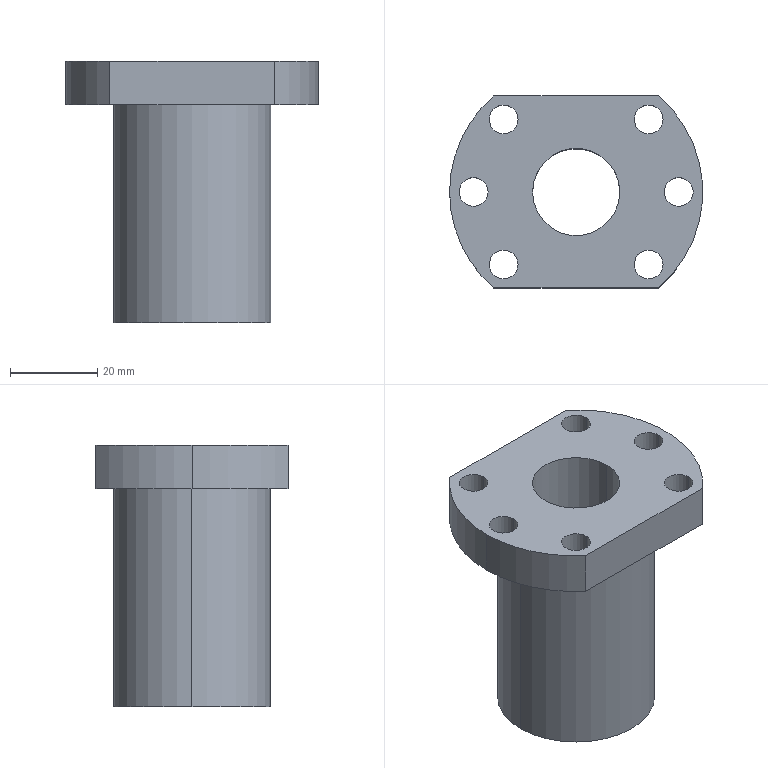Part | STEP file | SM140A-20-1140D-Slide plate 140-1000 -1000-2 | 1 solid | 24 faces | box 58 x 44 x 60 mm | volume 52790 mm3 | cylinder 19 | plane 5 | commonest cylinder face diameters 6.6 x12 58 x3 20 x2 36 x2